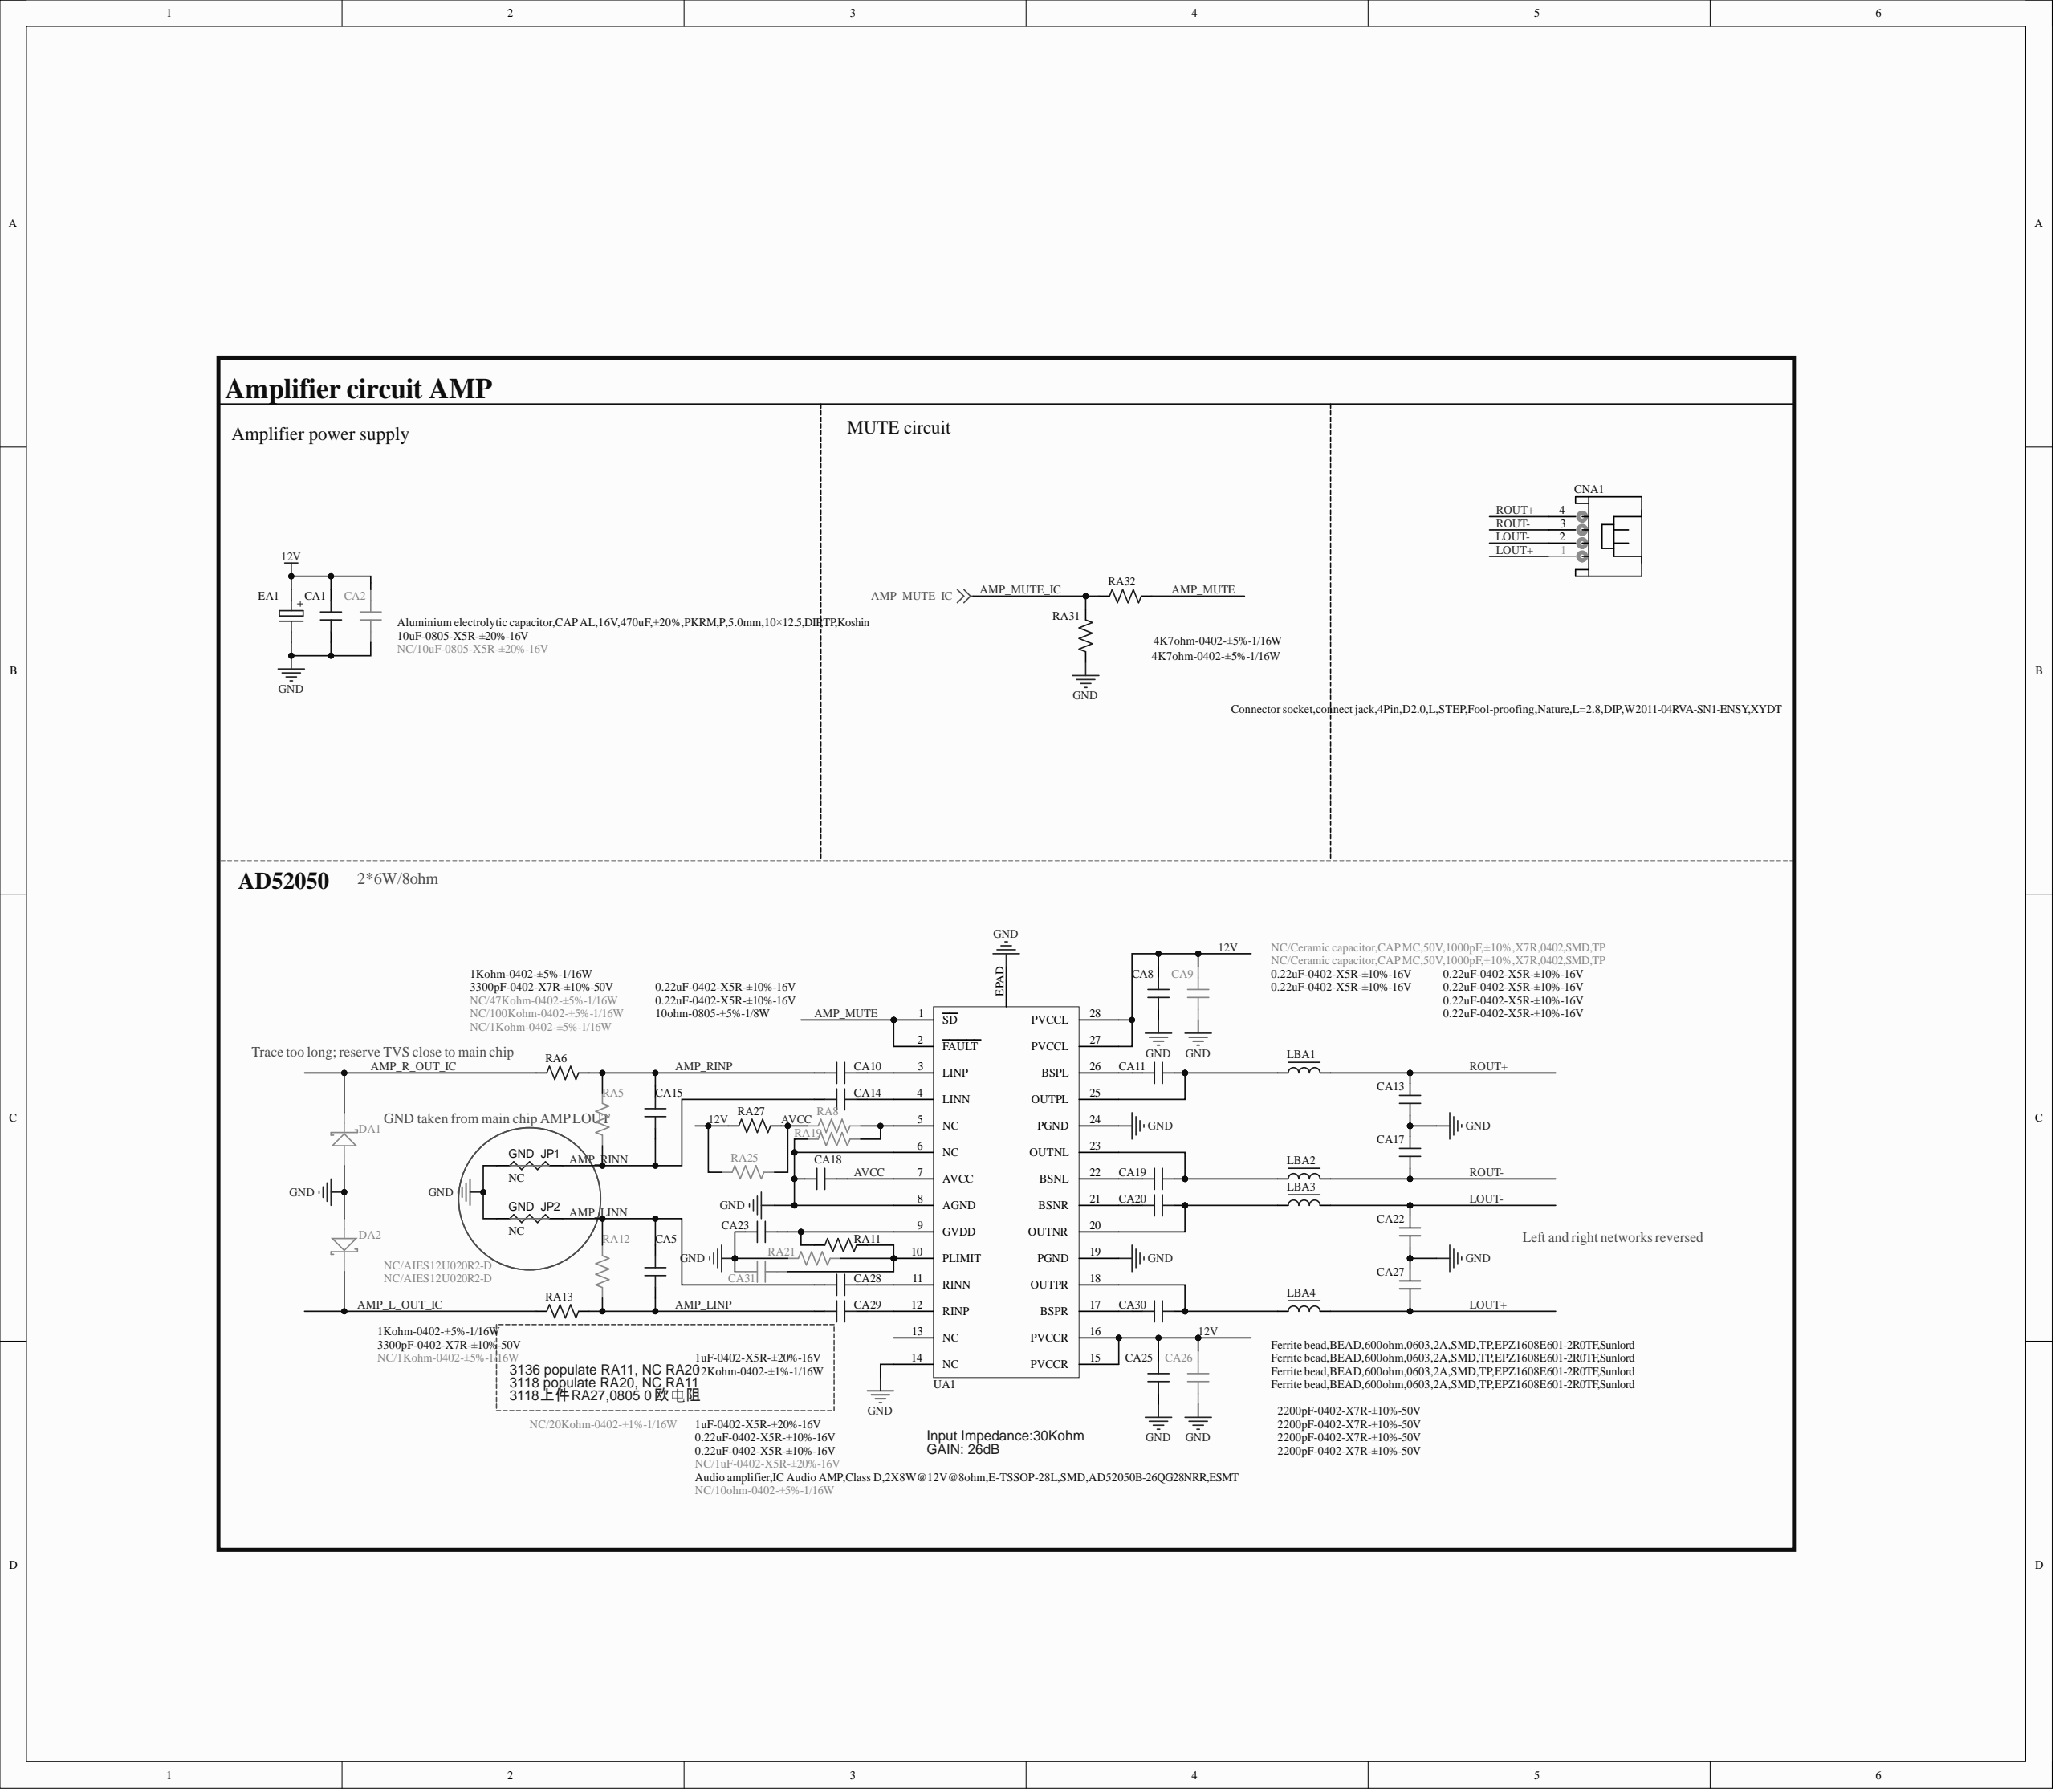Circuit board | Altium Designer | 951 parts | 509 nets | one sheet of the schematic
Parts on this sheet (reference | value | footprint):
CA1 | 10uF-0805-X5R-±20%-16V | C0805
CA2 | NC/10uF-0805-X5R-±20%-16V | C0805
CA5 | 3300pF-0402-X7R-±10%-50V | C0402
CA8 | 0.22uF-0402-X5R-±10%-16V | C0402
CA9 | NC/Ceramic capacitor,CAP MC,50V,1000pF,±10%,X7R,0402,SMD,TP | C0402
CA10 | 0.22uF-0402-X5R-±10%-16V | C0402
CA11 | 0.22uF-0402-X5R-±10%-16V | C0402
CA13 | 2200pF-0402-X7R-±10%-50V | C0402
CA14 | 0.22uF-0402-X5R-±10%-16V | C0402
CA15 | 3300pF-0402-X7R-±10%-50V | C0402
CA17 | 2200pF-0402-X7R-±10%-50V | C0402
CA18 | 1uF-0402-X5R-±20%-16V | C0402
CA19 | 0.22uF-0402-X5R-±10%-16V | C0402
CA20 | 0.22uF-0402-X5R-±10%-16V | C0402
CA22 | 2200pF-0402-X7R-±10%-50V | C0402
CA23 | 1uF-0402-X5R-±20%-16V | C0402
CA25 | 0.22uF-0402-X5R-±10%-16V | C0402
CA26 | NC/Ceramic capacitor,CAP MC,50V,1000pF,±10%,X7R,0402,SMD,TP | C0402
CA27 | 2200pF-0402-X7R-±10%-50V | C0402
CA28 | 0.22uF-0402-X5R-±10%-16V | C0402
CA29 | 0.22uF-0402-X5R-±10%-16V | C0402
CA30 | 0.22uF-0402-X5R-±10%-16V | C0402
CA31 | NC/1uF-0402-X5R-±20%-16V | C0402
CNA1 | Connector socket,connect jack,4Pin,D2.0,L,STEP,Fool-proofing,Nature,L=2.8,DIP,W2011-04RVA-SN1-ENSY,XYDT | SIP4H/2.0D-6
DA1 | NC/AIES12U020R2-D | DIODE-S0402
DA2 | NC/AIES12U020R2-D | DIODE-S0402
EA1 | Aluminium electrolytic capacitor,CAP AL,16V,470uF,±20%,PKRM,P,5.0mm,10×12.5,DIP,TP,Koshin | EC(10*12)-V-5
GND_JP1 | NC | GND
GND_JP2 | NC | GND
LBA1 | Ferrite bead,BEAD,600ohm,0603,2A,SMD,TP,EPZ1608E601-2R0TF,Sunlord | L0603
LBA2 | Ferrite bead,BEAD,600ohm,0603,2A,SMD,TP,EPZ1608E601-2R0TF,Sunlord | L0603
LBA3 | Ferrite bead,BEAD,600ohm,0603,2A,SMD,TP,EPZ1608E601-2R0TF,Sunlord | L0603
LBA4 | Ferrite bead,BEAD,600ohm,0603,2A,SMD,TP,EPZ1608E601-2R0TF,Sunlord | L0603
RA5 | NC/1Kohm-0402-±5%-1/16W | R0402
RA6 | 1Kohm-0402-±5%-1/16W | R0402
RA8 | NC/100Kohm-0402-±5%-1/16W | R0402
RA11 | 12Kohm-0402-±1%-1/16W | R0402
RA12 | NC/1Kohm-0402-±5%-1/16W | R0402
RA13 | 1Kohm-0402-±5%-1/16W | R0402
RA19 | NC/47Kohm-0402-±5%-1/16W | R0402
RA21 | NC/20Kohm-0402-±1%-1/16W | R0402
RA25 | NC/10ohm-0402-±5%-1/16W | R0402
RA27 | 10ohm-0805-±5%-1/8W | R0805
RA31 | 4K7ohm-0402-±5%-1/16W | R0402
RA32 | 4K7ohm-0402-±5%-1/16W | R0402
UA1 | Audio amplifier,IC Audio AMP,Class D,2X8W@12V@8ohm,E-TSSOP-28L,SMD,AD52050B-26QG28NRR,ESMT | SOP28/0.65-7
Nets of these parts (net: part-pin ...):
ROUT-: CA17-1 CNA1-3 LBA2-2
ROUT+: CA13-2 CNA1-4 LBA1-2
NetRA8_2: RA8-2 RA19-2 UA1-5
NetCA31_1: CA31-1 RA11-2 RA21-2 UA1-10
NetCA30_2: CA30-2 UA1-17
NetCA30_1: CA30-1 LBA4-1 UA1-18
NetCA29_1: CA29-1 UA1-12
NetCA28_1: CA28-1 UA1-11
NetCA23_1: CA23-1 RA11-1 UA1-9
NetCA20_2: CA20-2 UA1-21
NetCA20_1: CA20-1 LBA3-1 UA1-20
NetCA19_2: CA19-2 UA1-22
NetCA19_1: CA19-1 LBA2-1 UA1-23
NetCA14_1: CA14-1 UA1-4
NetCA11_2: CA11-2 UA1-26
NetCA11_1: CA11-1 LBA1-1 UA1-25
NetCA10_1: CA10-1 UA1-3
LOUT-: CA22-2 CNA1-2 LBA3-2
LOUT+: CA27-1 CNA1-1 LBA4-2
GND: CA1-1 CA2-1 CA8-1 CA9-1 CA13-1 CA17-2 CA18-2 CA22-1 CA23-2 CA25-2 CA26-1 CA27-2 CA31-2 DA1-A DA2-A EA1-2 GND_JP1-JP_2K GND_JP2-JP_2K RA19-1 RA21-1 RA31-1 UA1-6 UA1-8 UA1-14 UA1-19 UA1-24 UA1-EPAD
AVCC: CA18-1 RA8-1 RA25-2 RA27-2 UA1-7
AMP_RINP: CA10-2 CA15-2 RA5-2 RA6-2
AMP_RINN: CA14-2 CA15-1 GND_JP1-JP_1K RA5-1
AMP_R_OUT_IC: DA1-K RA6-1
AMP_MUTE_IC: RA31-2 RA32-2
AMP_MUTE: RA32-1 UA1-1 UA1-2
AMP_LINP: CA5-1 CA29-2 RA12-1 RA13-2
AMP_LINN: CA5-2 CA28-2 GND_JP2-JP_1K RA12-2
AMP_L_OUT_IC: DA2-K RA13-1
12V: CA1-2 CA2-2 CA8-2 CA9-2 CA25-1 CA26-2 EA1-1 RA25-1 RA27-1 UA1-15 UA1-16 UA1-27 UA1-28